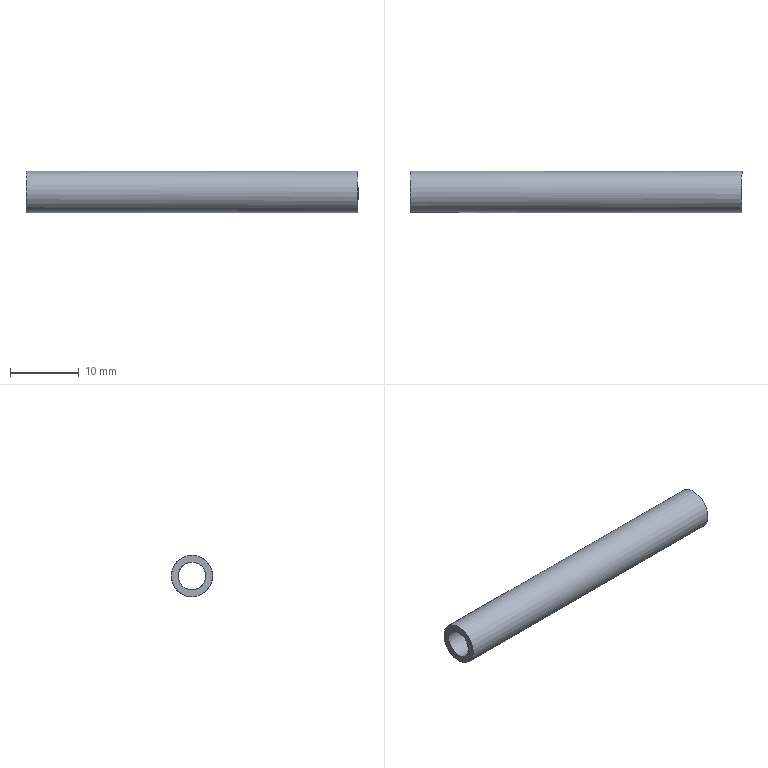Part | NX | features solid 2 | 1 solid | 4 faces | box 48.205 x 6 x 6 mm | volume 757.196 mm3 | cylinder 2 | plane 2 | commonest cylinder face diameters 4 x1 6 x1
STEP:
#1=CARTESIAN_POINT('',(-123.205,-115.,345.));
#2=VERTEX_POINT('',#1);
#3=CARTESIAN_POINT('',(-123.205,-115.,347.));
#4=DIRECTION('',(1.,0.,0.));
#5=DIRECTION('',(0.,0.,-1.));
#6=AXIS2_PLACEMENT_3D('',#3,#4,#5);
#7=CIRCLE('',#6,2.);
#8=EDGE_CURVE('',#2,#2,#7,.F.);
#9=ORIENTED_EDGE('',*,*,#8,.T.);
#10=EDGE_LOOP('',(#9));
#11=FACE_BOUND('',#10,.T.);
#12=CARTESIAN_POINT('',(-75.,-117.,347.));
#13=VERTEX_POINT('',#12);
#14=CARTESIAN_POINT('',(-75.,-115.,347.));
#15=DIRECTION('',(-1.,0.,0.));
#16=DIRECTION('',(0.,-1.,0.));
#17=AXIS2_PLACEMENT_3D('',#14,#15,#16);
#18=CIRCLE('',#17,2.);
#19=EDGE_CURVE('',#13,#13,#18,.T.);
#20=ORIENTED_EDGE('',*,*,#19,.F.);
#21=EDGE_LOOP('',(#20));
#22=FACE_BOUND('',#21,.T.);
#23=CARTESIAN_POINT('',(-273.824,-115.,347.));
#24=DIRECTION('',(1.,0.,0.));
#25=DIRECTION('',(0.,1.,0.));
#26=AXIS2_PLACEMENT_3D('',#23,#24,#25);
#27=CYLINDRICAL_SURFACE('',#26,2.);
#28=ADVANCED_FACE('',(#11,#22),#27,.F.);
#29=CARTESIAN_POINT('',(-123.205,-115.,344.));
#30=VERTEX_POINT('',#29);
#31=CARTESIAN_POINT('',(-123.205,-115.,347.));
#32=DIRECTION('',(1.,0.,0.));
#33=DIRECTION('',(0.,0.,-1.));
#34=AXIS2_PLACEMENT_3D('',#31,#32,#33);
#35=CIRCLE('',#34,3.);
#36=EDGE_CURVE('',#30,#30,#35,.F.);
#37=ORIENTED_EDGE('',*,*,#36,.F.);
#38=EDGE_LOOP('',(#37));
#39=FACE_BOUND('',#38,.T.);
#40=CARTESIAN_POINT('',(-75.,-118.,347.));
#41=VERTEX_POINT('',#40);
#42=CARTESIAN_POINT('',(-75.,-115.,347.));
#43=DIRECTION('',(-1.,0.,0.));
#44=DIRECTION('',(0.,-1.,0.));
#45=AXIS2_PLACEMENT_3D('',#42,#43,#44);
#46=CIRCLE('',#45,3.);
#47=EDGE_CURVE('',#41,#41,#46,.T.);
#48=ORIENTED_EDGE('',*,*,#47,.T.);
#49=EDGE_LOOP('',(#48));
#50=FACE_BOUND('',#49,.T.);
#51=CARTESIAN_POINT('',(-273.824,-115.,347.));
#52=DIRECTION('',(1.,0.,0.));
#53=DIRECTION('',(0.,1.,0.));
#54=AXIS2_PLACEMENT_3D('',#51,#52,#53);
#55=CYLINDRICAL_SURFACE('',#54,3.);
#56=ADVANCED_FACE('',(#39,#50),#55,.T.);
#57=ORIENTED_EDGE('',*,*,#8,.F.);
#58=EDGE_LOOP('',(#57));
#59=FACE_BOUND('',#58,.T.);
#60=ORIENTED_EDGE('',*,*,#36,.T.);
#61=EDGE_LOOP('',(#60));
#62=FACE_BOUND('',#61,.T.);
#63=CARTESIAN_POINT('',(-123.205,-140.535,126.));
#64=DIRECTION('',(1.,0.,0.));
#65=DIRECTION('',(0.,1.,0.));
#66=AXIS2_PLACEMENT_3D('',#63,#64,#65);
#67=PLANE('',#66);
#68=ADVANCED_FACE('',(#59,#62),#67,.F.);
#69=ORIENTED_EDGE('',*,*,#19,.T.);
#70=EDGE_LOOP('',(#69));
#71=FACE_BOUND('',#70,.T.);
#72=ORIENTED_EDGE('',*,*,#47,.F.);
#73=EDGE_LOOP('',(#72));
#74=FACE_BOUND('',#73,.T.);
#75=CARTESIAN_POINT('',(-75.,-115.,347.));
#76=DIRECTION('',(-1.,0.,0.));
#77=DIRECTION('',(0.,-1.,0.));
#78=AXIS2_PLACEMENT_3D('',#75,#76,#77);
#79=PLANE('',#78);
#80=ADVANCED_FACE('',(#71,#74),#79,.F.);
#81=CLOSED_SHELL('',(#28,#56,#68,#80));
#82=MANIFOLD_SOLID_BREP('',#81);
#83=(LENGTH_UNIT()NAMED_UNIT(*)SI_UNIT(.MILLI.,.METRE.));
#84=UNCERTAINTY_MEASURE_WITH_UNIT(LENGTH_MEASURE(0.00001),#83,'','');
#85=(NAMED_UNIT(*)PLANE_ANGLE_UNIT()SI_UNIT($,.RADIAN.));
#86=(NAMED_UNIT(*)SI_UNIT($,.STERADIAN.)SOLID_ANGLE_UNIT());
#87=(GEOMETRIC_REPRESENTATION_CONTEXT(3)GLOBAL_UNCERTAINTY_ASSIGNED_CONTEXT((#84))GLOBAL_UNIT_ASSIGNED_CONTEXT((#83,#85,#86))REPRESENTATION_CONTEXT('',''));
#88=ADVANCED_BREP_SHAPE_REPRESENTATION('',(#82),#87);